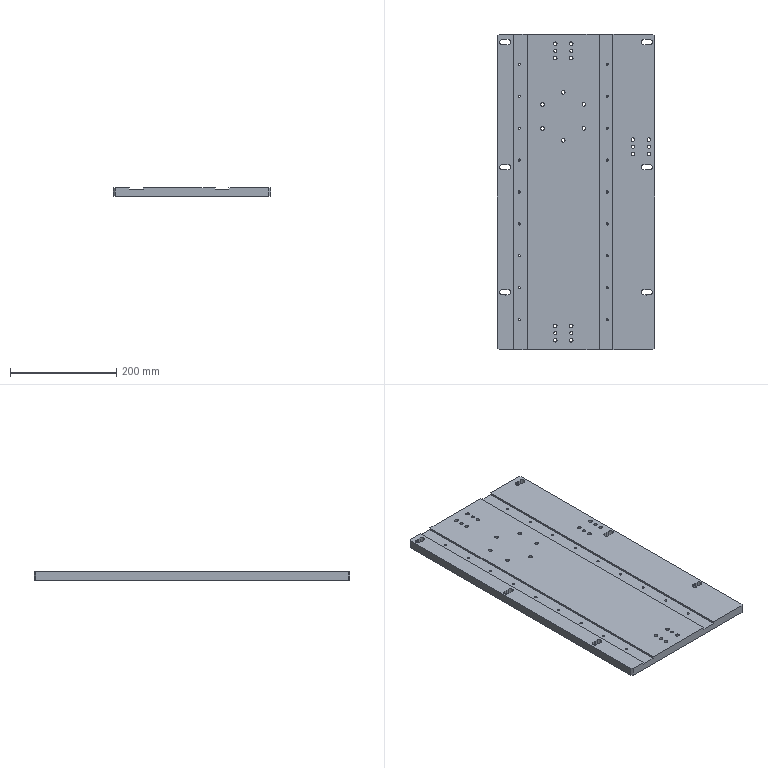Part | SolidWorks | features HoleWzd 6, ICE 2, Chamfer 1, Cut 1, Extrusion 1 | 1 solid | 156 faces | box 295 x 593 x 16 mm | volume 2656346 mm3 | cylinder 114 | plane 42 | commonest cylinder face diameters 4.2 x36 6.8 x36 10 x18 6 x12 10.1 x12